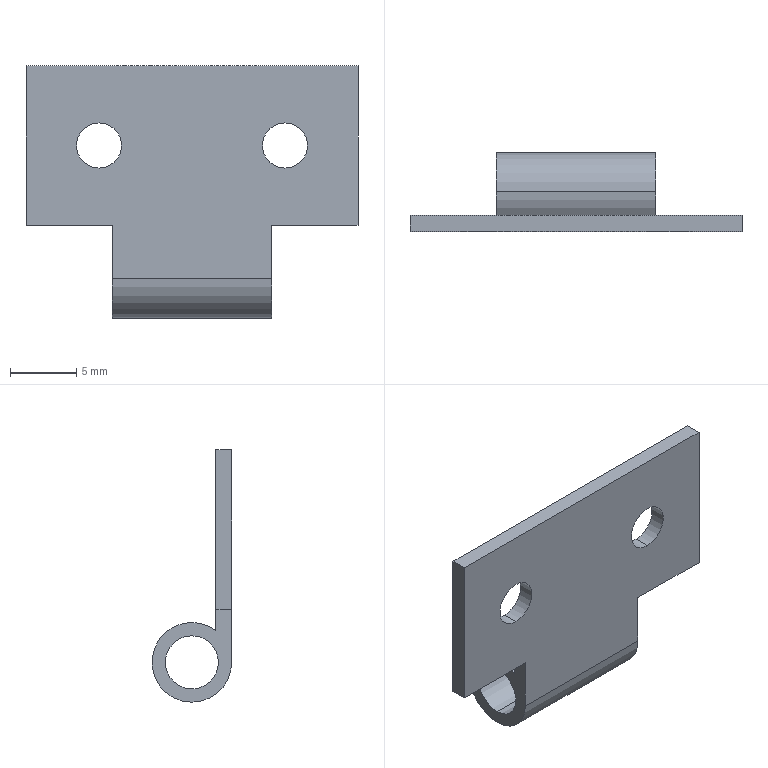Part | SolidWorks | features ICE 2, Extrusion 1, MirrorPattern 1 | 1 solid | 18 faces | box 25 x 6 x 19 mm | volume 560.152 mm3 | cylinder 9 | plane 9 | commonest cylinder face diameters 3.4 x4 6 x3 4 x2
STEP:
#1=CARTESIAN_POINT('',(-7.,-3.,8.3));
#2=VERTEX_POINT('',#1);
#3=CARTESIAN_POINT('',(-7.,-3.,11.7));
#4=VERTEX_POINT('',#3);
#5=CARTESIAN_POINT('',(-7.,-3.,10.));
#6=DIRECTION('',(0.,1.,0.));
#7=DIRECTION('',(0.,0.,1.));
#8=AXIS2_PLACEMENT_3D('',#5,#6,#7);
#9=CIRCLE('',#8,1.7);
#10=EDGE_CURVE('',#2,#4,#9,.T.);
#11=ORIENTED_EDGE('',*,*,#10,.F.);
#12=CARTESIAN_POINT('',(-7.,-1.8,8.3));
#13=VERTEX_POINT('',#12);
#14=CARTESIAN_POINT('',(-7.,-3.,8.3));
#15=DIRECTION('',(0.,1.,0.));
#16=VECTOR('',#15,1000.);
#17=LINE('',#14,#16);
#18=EDGE_CURVE('',#2,#13,#17,.T.);
#19=ORIENTED_EDGE('',*,*,#18,.T.);
#20=CARTESIAN_POINT('',(-7.,-1.8,11.7));
#21=VERTEX_POINT('',#20);
#22=CARTESIAN_POINT('',(-7.,-1.8,10.));
#23=DIRECTION('',(0.,1.,0.));
#24=DIRECTION('',(0.,0.,1.));
#25=AXIS2_PLACEMENT_3D('',#22,#23,#24);
#26=CIRCLE('',#25,1.7);
#27=EDGE_CURVE('',#13,#21,#26,.T.);
#28=ORIENTED_EDGE('',*,*,#27,.T.);
#29=CARTESIAN_POINT('',(-7.,-3.,11.7));
#30=DIRECTION('',(0.,1.,0.));
#31=VECTOR('',#30,1000.);
#32=LINE('',#29,#31);
#33=EDGE_CURVE('',#4,#21,#32,.T.);
#34=ORIENTED_EDGE('',*,*,#33,.F.);
#35=EDGE_LOOP('',(#11,#19,#28,#34));
#36=FACE_OUTER_BOUND('',#35,.T.);
#37=CARTESIAN_POINT('',(-7.,-3.,10.));
#38=DIRECTION('',(0.,1.,0.));
#39=DIRECTION('',(0.,0.,1.));
#40=AXIS2_PLACEMENT_3D('',#37,#38,#39);
#41=CYLINDRICAL_SURFACE('',#40,1.7);
#42=ADVANCED_FACE('',(#36),#41,.F.);
#43=CARTESIAN_POINT('',(7.,-3.,8.3));
#44=VERTEX_POINT('',#43);
#45=CARTESIAN_POINT('',(7.,-3.,11.7));
#46=VERTEX_POINT('',#45);
#47=CARTESIAN_POINT('',(7.,-3.,10.));
#48=DIRECTION('',(0.,1.,0.));
#49=DIRECTION('',(0.,0.,1.));
#50=AXIS2_PLACEMENT_3D('',#47,#48,#49);
#51=CIRCLE('',#50,1.7);
#52=EDGE_CURVE('',#44,#46,#51,.T.);
#53=ORIENTED_EDGE('',*,*,#52,.F.);
#54=CARTESIAN_POINT('',(7.,-1.8,8.3));
#55=VERTEX_POINT('',#54);
#56=CARTESIAN_POINT('',(7.,-3.,8.3));
#57=DIRECTION('',(0.,1.,0.));
#58=VECTOR('',#57,1000.);
#59=LINE('',#56,#58);
#60=EDGE_CURVE('',#44,#55,#59,.T.);
#61=ORIENTED_EDGE('',*,*,#60,.T.);
#62=CARTESIAN_POINT('',(7.,-1.8,11.7));
#63=VERTEX_POINT('',#62);
#64=CARTESIAN_POINT('',(7.,-1.8,10.));
#65=DIRECTION('',(0.,1.,0.));
#66=DIRECTION('',(0.,0.,1.));
#67=AXIS2_PLACEMENT_3D('',#64,#65,#66);
#68=CIRCLE('',#67,1.7);
#69=EDGE_CURVE('',#55,#63,#68,.T.);
#70=ORIENTED_EDGE('',*,*,#69,.T.);
#71=CARTESIAN_POINT('',(7.,-3.,11.7));
#72=DIRECTION('',(0.,1.,0.));
#73=VECTOR('',#72,1000.);
#74=LINE('',#71,#73);
#75=EDGE_CURVE('',#46,#63,#74,.T.);
#76=ORIENTED_EDGE('',*,*,#75,.F.);
#77=EDGE_LOOP('',(#53,#61,#70,#76));
#78=FACE_OUTER_BOUND('',#77,.T.);
#79=CARTESIAN_POINT('',(7.,-3.,10.));
#80=DIRECTION('',(0.,1.,0.));
#81=DIRECTION('',(0.,0.,1.));
#82=AXIS2_PLACEMENT_3D('',#79,#80,#81);
#83=CYLINDRICAL_SURFACE('',#82,1.7);
#84=ADVANCED_FACE('',(#78),#83,.F.);
#85=CARTESIAN_POINT('',(6.,0.,2.));
#86=VERTEX_POINT('',#85);
#87=CARTESIAN_POINT('',(6.,0.,-2.));
#88=VERTEX_POINT('',#87);
#89=CARTESIAN_POINT('',(6.,0.,0.));
#90=DIRECTION('',(1.,0.,0.));
#91=DIRECTION('',(0.,0.,-1.));
#92=AXIS2_PLACEMENT_3D('',#89,#90,#91);
#93=CIRCLE('',#92,2.);
#94=EDGE_CURVE('',#86,#88,#93,.T.);
#95=ORIENTED_EDGE('',*,*,#94,.T.);
#96=CARTESIAN_POINT('',(-6.,0.,-2.));
#97=VERTEX_POINT('',#96);
#98=CARTESIAN_POINT('',(12.5,0.,-2.));
#99=DIRECTION('',(-1.,0.,0.));
#100=VECTOR('',#99,1000.);
#101=LINE('',#98,#100);
#102=EDGE_CURVE('',#88,#97,#101,.T.);
#103=ORIENTED_EDGE('',*,*,#102,.T.);
#104=CARTESIAN_POINT('',(-6.,0.,2.));
#105=VERTEX_POINT('',#104);
#106=CARTESIAN_POINT('',(-6.,0.,0.));
#107=DIRECTION('',(-1.,0.,0.));
#108=DIRECTION('',(0.,0.,1.));
#109=AXIS2_PLACEMENT_3D('',#106,#107,#108);
#110=CIRCLE('',#109,2.);
#111=EDGE_CURVE('',#97,#105,#110,.T.);
#112=ORIENTED_EDGE('',*,*,#111,.T.);
#113=CARTESIAN_POINT('',(12.5,0.,2.));
#114=DIRECTION('',(-1.,0.,0.));
#115=VECTOR('',#114,1000.);
#116=LINE('',#113,#115);
#117=EDGE_CURVE('',#86,#105,#116,.T.);
#118=ORIENTED_EDGE('',*,*,#117,.F.);
#119=EDGE_LOOP('',(#95,#103,#112,#118));
#120=FACE_OUTER_BOUND('',#119,.T.);
#121=CARTESIAN_POINT('',(12.5,0.,0.));
#122=DIRECTION('',(-1.,0.,0.));
#123=DIRECTION('',(0.,0.,1.));
#124=AXIS2_PLACEMENT_3D('',#121,#122,#123);
#125=CYLINDRICAL_SURFACE('',#124,2.);
#126=ADVANCED_FACE('',(#120),#125,.F.);
#127=CARTESIAN_POINT('',(6.,0.,-3.));
#128=VERTEX_POINT('',#127);
#129=CARTESIAN_POINT('',(6.,0.,3.));
#130=VERTEX_POINT('',#129);
#131=CARTESIAN_POINT('',(6.,0.,0.));
#132=DIRECTION('',(1.,0.,0.));
#133=DIRECTION('',(0.,0.,-1.));
#134=AXIS2_PLACEMENT_3D('',#131,#132,#133);
#135=CIRCLE('',#134,3.);
#136=EDGE_CURVE('',#128,#130,#135,.T.);
#137=ORIENTED_EDGE('',*,*,#136,.F.);
#138=CARTESIAN_POINT('',(-6.,0.,-3.));
#139=VERTEX_POINT('',#138);
#140=CARTESIAN_POINT('',(12.5,0.,-3.));
#141=DIRECTION('',(-1.,0.,0.));
#142=VECTOR('',#141,1000.);
#143=LINE('',#140,#142);
#144=EDGE_CURVE('',#128,#139,#143,.T.);
#145=ORIENTED_EDGE('',*,*,#144,.T.);
#146=CARTESIAN_POINT('',(-6.,0.,3.));
#147=VERTEX_POINT('',#146);
#148=CARTESIAN_POINT('',(-6.,0.,0.));
#149=DIRECTION('',(1.,0.,0.));
#150=DIRECTION('',(0.,0.,-1.));
#151=AXIS2_PLACEMENT_3D('',#148,#149,#150);
#152=CIRCLE('',#151,3.);
#153=EDGE_CURVE('',#139,#147,#152,.T.);
#154=ORIENTED_EDGE('',*,*,#153,.T.);
#155=CARTESIAN_POINT('',(12.5,0.,3.));
#156=DIRECTION('',(-1.,0.,0.));
#157=VECTOR('',#156,1000.);
#158=LINE('',#155,#157);
#159=EDGE_CURVE('',#130,#147,#158,.T.);
#160=ORIENTED_EDGE('',*,*,#159,.F.);
#161=EDGE_LOOP('',(#137,#145,#154,#160));
#162=FACE_OUTER_BOUND('',#161,.T.);
#163=CARTESIAN_POINT('',(12.5,0.,0.));
#164=DIRECTION('',(-1.,0.,0.));
#165=DIRECTION('',(0.,0.,1.));
#166=AXIS2_PLACEMENT_3D('',#163,#164,#165);
#167=CYLINDRICAL_SURFACE('',#166,3.);
#168=ADVANCED_FACE('',(#162),#167,.T.);
#169=CARTESIAN_POINT('',(6.,-1.8,2.4));
#170=VERTEX_POINT('',#169);
#171=CARTESIAN_POINT('',(6.,0.,0.));
#172=DIRECTION('',(1.,0.,0.));
#173=DIRECTION('',(0.,0.,-1.));
#174=AXIS2_PLACEMENT_3D('',#171,#172,#173);
#175=CIRCLE('',#174,3.);
#176=EDGE_CURVE('',#130,#170,#175,.T.);
#177=ORIENTED_EDGE('',*,*,#176,.F.);
#178=ORIENTED_EDGE('',*,*,#159,.T.);
#179=CARTESIAN_POINT('',(-6.,-1.8,2.4));
#180=VERTEX_POINT('',#179);
#181=CARTESIAN_POINT('',(-6.,0.,0.));
#182=DIRECTION('',(1.,0.,0.));
#183=DIRECTION('',(0.,0.,-1.));
#184=AXIS2_PLACEMENT_3D('',#181,#182,#183);
#185=CIRCLE('',#184,3.);
#186=EDGE_CURVE('',#147,#180,#185,.T.);
#187=ORIENTED_EDGE('',*,*,#186,.T.);
#188=CARTESIAN_POINT('',(12.5,-1.8,2.4));
#189=DIRECTION('',(-1.,0.,0.));
#190=VECTOR('',#189,1000.);
#191=LINE('',#188,#190);
#192=EDGE_CURVE('',#170,#180,#191,.T.);
#193=ORIENTED_EDGE('',*,*,#192,.F.);
#194=EDGE_LOOP('',(#177,#178,#187,#193));
#195=FACE_OUTER_BOUND('',#194,.T.);
#196=CARTESIAN_POINT('',(12.5,0.,0.));
#197=DIRECTION('',(-1.,0.,0.));
#198=DIRECTION('',(0.,0.,1.));
#199=AXIS2_PLACEMENT_3D('',#196,#197,#198);
#200=CYLINDRICAL_SURFACE('',#199,3.);
#201=ADVANCED_FACE('',(#195),#200,.T.);
#202=ORIENTED_EDGE('',*,*,#144,.F.);
#203=CARTESIAN_POINT('',(6.,-3.,0.));
#204=VERTEX_POINT('',#203);
#205=CARTESIAN_POINT('',(6.,0.,0.));
#206=DIRECTION('',(1.,0.,0.));
#207=DIRECTION('',(0.,0.,-1.));
#208=AXIS2_PLACEMENT_3D('',#205,#206,#207);
#209=CIRCLE('',#208,3.);
#210=EDGE_CURVE('',#204,#128,#209,.T.);
#211=ORIENTED_EDGE('',*,*,#210,.F.);
#212=CARTESIAN_POINT('',(-6.,-3.,0.));
#213=VERTEX_POINT('',#212);
#214=CARTESIAN_POINT('',(12.5,-3.,0.));
#215=DIRECTION('',(-1.,0.,0.));
#216=VECTOR('',#215,1000.);
#217=LINE('',#214,#216);
#218=EDGE_CURVE('',#204,#213,#217,.T.);
#219=ORIENTED_EDGE('',*,*,#218,.T.);
#220=CARTESIAN_POINT('',(-6.,0.,0.));
#221=DIRECTION('',(1.,0.,0.));
#222=DIRECTION('',(0.,0.,-1.));
#223=AXIS2_PLACEMENT_3D('',#220,#221,#222);
#224=CIRCLE('',#223,3.);
#225=EDGE_CURVE('',#213,#139,#224,.T.);
#226=ORIENTED_EDGE('',*,*,#225,.T.);
#227=EDGE_LOOP('',(#202,#211,#219,#226));
#228=FACE_OUTER_BOUND('',#227,.T.);
#229=CARTESIAN_POINT('',(12.5,0.,0.));
#230=DIRECTION('',(-1.,0.,0.));
#231=DIRECTION('',(0.,0.,1.));
#232=AXIS2_PLACEMENT_3D('',#229,#230,#231);
#233=CYLINDRICAL_SURFACE('',#232,3.);
#234=ADVANCED_FACE('',(#228),#233,.T.);
#235=ORIENTED_EDGE('',*,*,#102,.F.);
#236=CARTESIAN_POINT('',(6.,0.,0.));
#237=DIRECTION('',(1.,0.,0.));
#238=DIRECTION('',(0.,0.,-1.));
#239=AXIS2_PLACEMENT_3D('',#236,#237,#238);
#240=CIRCLE('',#239,2.);
#241=EDGE_CURVE('',#88,#86,#240,.T.);
#242=ORIENTED_EDGE('',*,*,#241,.T.);
#243=ORIENTED_EDGE('',*,*,#117,.T.);
#244=CARTESIAN_POINT('',(-6.,0.,0.));
#245=DIRECTION('',(-1.,0.,0.));
#246=DIRECTION('',(0.,0.,1.));
#247=AXIS2_PLACEMENT_3D('',#244,#245,#246);
#248=CIRCLE('',#247,2.);
#249=EDGE_CURVE('',#105,#97,#248,.T.);
#250=ORIENTED_EDGE('',*,*,#249,.T.);
#251=EDGE_LOOP('',(#235,#242,#243,#250));
#252=FACE_OUTER_BOUND('',#251,.T.);
#253=CARTESIAN_POINT('',(12.5,0.,0.));
#254=DIRECTION('',(-1.,0.,0.));
#255=DIRECTION('',(0.,0.,1.));
#256=AXIS2_PLACEMENT_3D('',#253,#254,#255);
#257=CYLINDRICAL_SURFACE('',#256,2.);
#258=ADVANCED_FACE('',(#252),#257,.F.);
#259=CARTESIAN_POINT('',(-12.5,-1.8,4.));
#260=VERTEX_POINT('',#259);
#261=CARTESIAN_POINT('',(-12.5,-3.,4.));
#262=VERTEX_POINT('',#261);
#263=CARTESIAN_POINT('',(-12.5,-1.8,4.));
#264=DIRECTION('',(0.,-1.,0.));
#265=VECTOR('',#264,1000.);
#266=LINE('',#263,#265);
#267=EDGE_CURVE('',#260,#262,#266,.T.);
#268=ORIENTED_EDGE('',*,*,#267,.T.);
#269=CARTESIAN_POINT('',(-12.5,-3.,16.));
#270=VERTEX_POINT('',#269);
#271=CARTESIAN_POINT('',(-12.5,-3.,0.));
#272=DIRECTION('',(0.,0.,-1.));
#273=VECTOR('',#272,1000.);
#274=LINE('',#271,#273);
#275=EDGE_CURVE('',#270,#262,#274,.T.);
#276=ORIENTED_EDGE('',*,*,#275,.F.);
#277=CARTESIAN_POINT('',(-12.5,-1.8,16.));
#278=VERTEX_POINT('',#277);
#279=CARTESIAN_POINT('',(-12.5,-3.,16.));
#280=DIRECTION('',(0.,-1.,0.));
#281=VECTOR('',#280,1000.);
#282=LINE('',#279,#281);
#283=EDGE_CURVE('',#278,#270,#282,.T.);
#284=ORIENTED_EDGE('',*,*,#283,.F.);
#285=CARTESIAN_POINT('',(-12.5,-1.8,16.));
#286=DIRECTION('',(0.,0.,1.));
#287=VECTOR('',#286,1000.);
#288=LINE('',#285,#287);
#289=EDGE_CURVE('',#260,#278,#288,.T.);
#290=ORIENTED_EDGE('',*,*,#289,.F.);
#291=EDGE_LOOP('',(#268,#276,#284,#290));
#292=FACE_OUTER_BOUND('',#291,.T.);
#293=CARTESIAN_POINT('',(-12.5,0.,0.));
#294=DIRECTION('',(1.,0.,0.));
#295=DIRECTION('',(0.,0.,-1.));
#296=AXIS2_PLACEMENT_3D('',#293,#294,#295);
#297=PLANE('',#296);
#298=ADVANCED_FACE('',(#292),#297,.F.);
#299=CARTESIAN_POINT('',(7.,-1.8,10.));
#300=DIRECTION('',(0.,1.,0.));
#301=DIRECTION('',(0.,0.,1.));
#302=AXIS2_PLACEMENT_3D('',#299,#300,#301);
#303=CIRCLE('',#302,1.7);
#304=EDGE_CURVE('',#63,#55,#303,.T.);
#305=ORIENTED_EDGE('',*,*,#304,.F.);
#306=ORIENTED_EDGE('',*,*,#69,.F.);
#307=EDGE_LOOP('',(#305,#306));
#308=FACE_BOUND('',#307,.T.);
#309=CARTESIAN_POINT('',(-7.,-1.8,10.));
#310=DIRECTION('',(0.,1.,0.));
#311=DIRECTION('',(0.,0.,1.));
#312=AXIS2_PLACEMENT_3D('',#309,#310,#311);
#313=CIRCLE('',#312,1.7);
#314=EDGE_CURVE('',#21,#13,#313,.T.);
#315=ORIENTED_EDGE('',*,*,#314,.F.);
#316=ORIENTED_EDGE('',*,*,#27,.F.);
#317=EDGE_LOOP('',(#315,#316));
#318=FACE_BOUND('',#317,.T.);
#319=CARTESIAN_POINT('',(-6.,-1.8,4.));
#320=VERTEX_POINT('',#319);
#321=CARTESIAN_POINT('',(-6.,-1.8,4.));
#322=DIRECTION('',(-1.,0.,0.));
#323=VECTOR('',#322,1000.);
#324=LINE('',#321,#323);
#325=EDGE_CURVE('',#320,#260,#324,.T.);
#326=ORIENTED_EDGE('',*,*,#325,.T.);
#327=ORIENTED_EDGE('',*,*,#289,.T.);
#328=CARTESIAN_POINT('',(12.5,-1.8,16.));
#329=VERTEX_POINT('',#328);
#330=CARTESIAN_POINT('',(12.5,-1.8,16.));
#331=DIRECTION('',(-1.,0.,0.));
#332=VECTOR('',#331,1000.);
#333=LINE('',#330,#332);
#334=EDGE_CURVE('',#329,#278,#333,.T.);
#335=ORIENTED_EDGE('',*,*,#334,.F.);
#336=CARTESIAN_POINT('',(12.5,-1.8,4.));
#337=VERTEX_POINT('',#336);
#338=CARTESIAN_POINT('',(12.5,-1.8,16.));
#339=DIRECTION('',(0.,0.,1.));
#340=VECTOR('',#339,1000.);
#341=LINE('',#338,#340);
#342=EDGE_CURVE('',#337,#329,#341,.T.);
#343=ORIENTED_EDGE('',*,*,#342,.F.);
#344=CARTESIAN_POINT('',(6.,-1.8,4.));
#345=VERTEX_POINT('',#344);
#346=CARTESIAN_POINT('',(6.,-1.8,4.));
#347=DIRECTION('',(1.,0.,0.));
#348=VECTOR('',#347,1000.);
#349=LINE('',#346,#348);
#350=EDGE_CURVE('',#345,#337,#349,.T.);
#351=ORIENTED_EDGE('',*,*,#350,.F.);
#352=CARTESIAN_POINT('',(6.,-1.8,2.4));
#353=DIRECTION('',(0.,0.,1.));
#354=VECTOR('',#353,1000.);
#355=LINE('',#352,#354);
#356=EDGE_CURVE('',#170,#345,#355,.T.);
#357=ORIENTED_EDGE('',*,*,#356,.F.);
#358=ORIENTED_EDGE('',*,*,#192,.T.);
#359=CARTESIAN_POINT('',(-6.,-1.8,2.4));
#360=DIRECTION('',(0.,0.,1.));
#361=VECTOR('',#360,1000.);
#362=LINE('',#359,#361);
#363=EDGE_CURVE('',#180,#320,#362,.T.);
#364=ORIENTED_EDGE('',*,*,#363,.T.);
#365=EDGE_LOOP('',(#326,#327,#335,#343,#351,#357,#358,#364));
#366=FACE_OUTER_BOUND('',#365,.T.);
#367=CARTESIAN_POINT('',(12.5,-1.8,16.));
#368=DIRECTION('',(0.,-1.,0.));
#369=DIRECTION('',(0.,0.,-1.));
#370=AXIS2_PLACEMENT_3D('',#367,#368,#369);
#371=PLANE('',#370);
#372=ADVANCED_FACE('',(#308,#318,#366),#371,.F.);
#373=CARTESIAN_POINT('',(7.,-3.,10.));
#374=DIRECTION('',(0.,1.,0.));
#375=DIRECTION('',(0.,0.,1.));
#376=AXIS2_PLACEMENT_3D('',#373,#374,#375);
#377=CIRCLE('',#376,1.7);
#378=EDGE_CURVE('',#46,#44,#377,.T.);
#379=ORIENTED_EDGE('',*,*,#378,.T.);
#380=ORIENTED_EDGE('',*,*,#52,.T.);
#381=EDGE_LOOP('',(#379,#380));
#382=FACE_BOUND('',#381,.T.);
#383=CARTESIAN_POINT('',(-7.,-3.,10.));
#384=DIRECTION('',(0.,1.,0.));
#385=DIRECTION('',(0.,0.,1.));
#386=AXIS2_PLACEMENT_3D('',#383,#384,#385);
#387=CIRCLE('',#386,1.7);
#388=EDGE_CURVE('',#4,#2,#387,.T.);
#389=ORIENTED_EDGE('',*,*,#388,.T.);
#390=ORIENTED_EDGE('',*,*,#10,.T.);
#391=EDGE_LOOP('',(#389,#390));
#392=FACE_BOUND('',#391,.T.);
#393=CARTESIAN_POINT('',(-6.,-3.,4.));
#394=VERTEX_POINT('',#393);
#395=CARTESIAN_POINT('',(-6.,-3.,4.));
#396=DIRECTION('',(-1.,0.,0.));
#397=VECTOR('',#396,1000.);
#398=LINE('',#395,#397);
#399=EDGE_CURVE('',#394,#262,#398,.T.);
#400=ORIENTED_EDGE('',*,*,#399,.F.);
#401=CARTESIAN_POINT('',(-6.,-3.,4.));
#402=DIRECTION('',(0.,0.,-1.));
#403=VECTOR('',#402,1000.);
#404=LINE('',#401,#403);
#405=EDGE_CURVE('',#394,#213,#404,.T.);
#406=ORIENTED_EDGE('',*,*,#405,.T.);
#407=ORIENTED_EDGE('',*,*,#218,.F.);
#408=CARTESIAN_POINT('',(6.,-3.,4.));
#409=VERTEX_POINT('',#408);
#410=CARTESIAN_POINT('',(6.,-3.,4.));
#411=DIRECTION('',(0.,0.,-1.));
#412=VECTOR('',#411,1000.);
#413=LINE('',#410,#412);
#414=EDGE_CURVE('',#409,#204,#413,.T.);
#415=ORIENTED_EDGE('',*,*,#414,.F.);
#416=CARTESIAN_POINT('',(12.5,-3.,4.));
#417=VERTEX_POINT('',#416);
#418=CARTESIAN_POINT('',(6.,-3.,4.));
#419=DIRECTION('',(1.,0.,0.));
#420=VECTOR('',#419,1000.);
#421=LINE('',#418,#420);
#422=EDGE_CURVE('',#409,#417,#421,.T.);
#423=ORIENTED_EDGE('',*,*,#422,.T.);
#424=CARTESIAN_POINT('',(12.5,-3.,16.));
#425=VERTEX_POINT('',#424);
#426=CARTESIAN_POINT('',(12.5,-3.,0.));
#427=DIRECTION('',(0.,0.,-1.));
#428=VECTOR('',#427,1000.);
#429=LINE('',#426,#428);
#430=EDGE_CURVE('',#425,#417,#429,.T.);
#431=ORIENTED_EDGE('',*,*,#430,.F.);
#432=CARTESIAN_POINT('',(12.5,-3.,16.));
#433=DIRECTION('',(-1.,0.,0.));
#434=VECTOR('',#433,1000.);
#435=LINE('',#432,#434);
#436=EDGE_CURVE('',#425,#270,#435,.T.);
#437=ORIENTED_EDGE('',*,*,#436,.T.);
#438=ORIENTED_EDGE('',*,*,#275,.T.);
#439=EDGE_LOOP('',(#400,#406,#407,#415,#423,#431,#437,#438));
#440=FACE_OUTER_BOUND('',#439,.T.);
#441=CARTESIAN_POINT('',(12.5,-3.,0.));
#442=DIRECTION('',(0.,1.,0.));
#443=DIRECTION('',(0.,0.,1.));
#444=AXIS2_PLACEMENT_3D('',#441,#442,#443);
#445=PLANE('',#444);
#446=ADVANCED_FACE('',(#382,#392,#440),#445,.F.);
#447=CARTESIAN_POINT('',(12.5,-1.8,4.));
#448=DIRECTION('',(0.,-1.,0.));
#449=VECTOR('',#448,1000.);
#450=LINE('',#447,#449);
#451=EDGE_CURVE('',#337,#417,#450,.T.);
#452=ORIENTED_EDGE('',*,*,#451,.F.);
#453=ORIENTED_EDGE('',*,*,#342,.T.);
#454=CARTESIAN_POINT('',(12.5,-3.,16.));
#455=DIRECTION('',(0.,-1.,0.));
#456=VECTOR('',#455,1000.);
#457=LINE('',#454,#456);
#458=EDGE_CURVE('',#329,#425,#457,.T.);
#459=ORIENTED_EDGE('',*,*,#458,.T.);
#460=ORIENTED_EDGE('',*,*,#430,.T.);
#461=EDGE_LOOP('',(#452,#453,#459,#460));
#462=FACE_OUTER_BOUND('',#461,.T.);
#463=CARTESIAN_POINT('',(12.5,0.,0.));
#464=DIRECTION('',(1.,0.,0.));
#465=DIRECTION('',(0.,0.,-1.));
#466=AXIS2_PLACEMENT_3D('',#463,#464,#465);
#467=PLANE('',#466);
#468=ADVANCED_FACE('',(#462),#467,.T.);
#469=ORIENTED_EDGE('',*,*,#283,.T.);
#470=ORIENTED_EDGE('',*,*,#436,.F.);
#471=ORIENTED_EDGE('',*,*,#458,.F.);
#472=ORIENTED_EDGE('',*,*,#334,.T.);
#473=EDGE_LOOP('',(#469,#470,#471,#472));
#474=FACE_OUTER_BOUND('',#473,.T.);
#475=CARTESIAN_POINT('',(12.5,-3.,16.));
#476=DIRECTION('',(0.,0.,-1.));
#477=DIRECTION('',(-1.,0.,0.));
#478=AXIS2_PLACEMENT_3D('',#475,#476,#477);
#479=PLANE('',#478);
#480=ADVANCED_FACE('',(#474),#479,.F.);
#481=ORIENTED_EDGE('',*,*,#60,.F.);
#482=ORIENTED_EDGE('',*,*,#378,.F.);
#483=ORIENTED_EDGE('',*,*,#75,.T.);
#484=ORIENTED_EDGE('',*,*,#304,.T.);
#485=EDGE_LOOP('',(#481,#482,#483,#484));
#486=FACE_OUTER_BOUND('',#485,.T.);
#487=CARTESIAN_POINT('',(7.,-3.,10.));
#488=DIRECTION('',(0.,1.,0.));
#489=DIRECTION('',(0.,0.,1.));
#490=AXIS2_PLACEMENT_3D('',#487,#488,#489);
#491=CYLINDRICAL_SURFACE('',#490,1.7);
#492=ADVANCED_FACE('',(#486),#491,.F.);
#493=ORIENTED_EDGE('',*,*,#18,.F.);
#494=ORIENTED_EDGE('',*,*,#388,.F.);
#495=ORIENTED_EDGE('',*,*,#33,.T.);
#496=ORIENTED_EDGE('',*,*,#314,.T.);
#497=EDGE_LOOP('',(#493,#494,#495,#496));
#498=FACE_OUTER_BOUND('',#497,.T.);
#499=CARTESIAN_POINT('',(-7.,-3.,10.));
#500=DIRECTION('',(0.,1.,0.));
#501=DIRECTION('',(0.,0.,1.));
#502=AXIS2_PLACEMENT_3D('',#499,#500,#501);
#503=CYLINDRICAL_SURFACE('',#502,1.7);
#504=ADVANCED_FACE('',(#498),#503,.F.);
#505=ORIENTED_EDGE('',*,*,#451,.T.);
#506=ORIENTED_EDGE('',*,*,#422,.F.);
#507=CARTESIAN_POINT('',(6.,-1.8,4.));
#508=DIRECTION('',(0.,-1.,0.));
#509=VECTOR('',#508,1000.);
#510=LINE('',#507,#509);
#511=EDGE_CURVE('',#345,#409,#510,.T.);
#512=ORIENTED_EDGE('',*,*,#511,.F.);
#513=ORIENTED_EDGE('',*,*,#350,.T.);
#514=EDGE_LOOP('',(#505,#506,#512,#513));
#515=FACE_OUTER_BOUND('',#514,.T.);
#516=CARTESIAN_POINT('',(6.,-1.8,4.));
#517=DIRECTION('',(0.,0.,1.));
#518=DIRECTION('',(1.,0.,0.));
#519=AXIS2_PLACEMENT_3D('',#516,#517,#518);
#520=PLANE('',#519);
#521=ADVANCED_FACE('',(#515),#520,.F.);
#522=ORIENTED_EDGE('',*,*,#94,.F.);
#523=ORIENTED_EDGE('',*,*,#241,.F.);
#524=EDGE_LOOP('',(#522,#523));
#525=FACE_BOUND('',#524,.T.);
#526=ORIENTED_EDGE('',*,*,#210,.T.);
#527=ORIENTED_EDGE('',*,*,#136,.T.);
#528=ORIENTED_EDGE('',*,*,#176,.T.);
#529=ORIENTED_EDGE('',*,*,#356,.T.);
#530=ORIENTED_EDGE('',*,*,#511,.T.);
#531=ORIENTED_EDGE('',*,*,#414,.T.);
#532=EDGE_LOOP('',(#526,#527,#528,#529,#530,#531));
#533=FACE_OUTER_BOUND('',#532,.T.);
#534=CARTESIAN_POINT('',(6.,0.,0.));
#535=DIRECTION('',(1.,0.,0.));
#536=DIRECTION('',(0.,0.,-1.));
#537=AXIS2_PLACEMENT_3D('',#534,#535,#536);
#538=PLANE('',#537);
#539=ADVANCED_FACE('',(#525,#533),#538,.T.);
#540=ORIENTED_EDGE('',*,*,#267,.F.);
#541=ORIENTED_EDGE('',*,*,#325,.F.);
#542=CARTESIAN_POINT('',(-6.,-1.8,4.));
#543=DIRECTION('',(0.,-1.,0.));
#544=VECTOR('',#543,1000.);
#545=LINE('',#542,#544);
#546=EDGE_CURVE('',#320,#394,#545,.T.);
#547=ORIENTED_EDGE('',*,*,#546,.T.);
#548=ORIENTED_EDGE('',*,*,#399,.T.);
#549=EDGE_LOOP('',(#540,#541,#547,#548));
#550=FACE_OUTER_BOUND('',#549,.T.);
#551=CARTESIAN_POINT('',(-6.,-1.8,4.));
#552=DIRECTION('',(0.,0.,-1.));
#553=DIRECTION('',(-1.,0.,0.));
#554=AXIS2_PLACEMENT_3D('',#551,#552,#553);
#555=PLANE('',#554);
#556=ADVANCED_FACE('',(#550),#555,.T.);
#557=ORIENTED_EDGE('',*,*,#249,.F.);
#558=ORIENTED_EDGE('',*,*,#111,.F.);
#559=EDGE_LOOP('',(#557,#558));
#560=FACE_BOUND('',#559,.T.);
#561=ORIENTED_EDGE('',*,*,#225,.F.);
#562=ORIENTED_EDGE('',*,*,#405,.F.);
#563=ORIENTED_EDGE('',*,*,#546,.F.);
#564=ORIENTED_EDGE('',*,*,#363,.F.);
#565=ORIENTED_EDGE('',*,*,#186,.F.);
#566=ORIENTED_EDGE('',*,*,#153,.F.);
#567=EDGE_LOOP('',(#561,#562,#563,#564,#565,#566));
#568=FACE_OUTER_BOUND('',#567,.T.);
#569=CARTESIAN_POINT('',(-6.,0.,0.));
#570=DIRECTION('',(-1.,0.,0.));
#571=DIRECTION('',(0.,0.,-1.));
#572=AXIS2_PLACEMENT_3D('',#569,#570,#571);
#573=PLANE('',#572);
#574=ADVANCED_FACE('',(#560,#568),#573,.T.);
#575=CLOSED_SHELL('',(#42,#84,#126,#168,#201,#234,#258,#298,#372,#446,#468,#480,#492,#504,#521,#539,#556,#574));
#576=MANIFOLD_SOLID_BREP('',#575);
#577=CARTESIAN_POINT('',(0.,0.,0.));
#578=DIRECTION('',(0.,0.,1.));
#579=DIRECTION('',(1.,0.,0.));
#580=AXIS2_PLACEMENT_3D('',#577,#578,#579);
#581=(LENGTH_UNIT()NAMED_UNIT(*)SI_UNIT(.MILLI.,.METRE.));
#582=UNCERTAINTY_MEASURE_WITH_UNIT(LENGTH_MEASURE(0.00001),#581,'','');
#583=(NAMED_UNIT(*)PLANE_ANGLE_UNIT()SI_UNIT($,.RADIAN.));
#584=(NAMED_UNIT(*)SI_UNIT($,.STERADIAN.)SOLID_ANGLE_UNIT());
#585=(GEOMETRIC_REPRESENTATION_CONTEXT(3)GLOBAL_UNCERTAINTY_ASSIGNED_CONTEXT((#582))GLOBAL_UNIT_ASSIGNED_CONTEXT((#581,#583,#584))REPRESENTATION_CONTEXT('',''));
#586=ADVANCED_BREP_SHAPE_REPRESENTATION('',(#576,#580),#585);